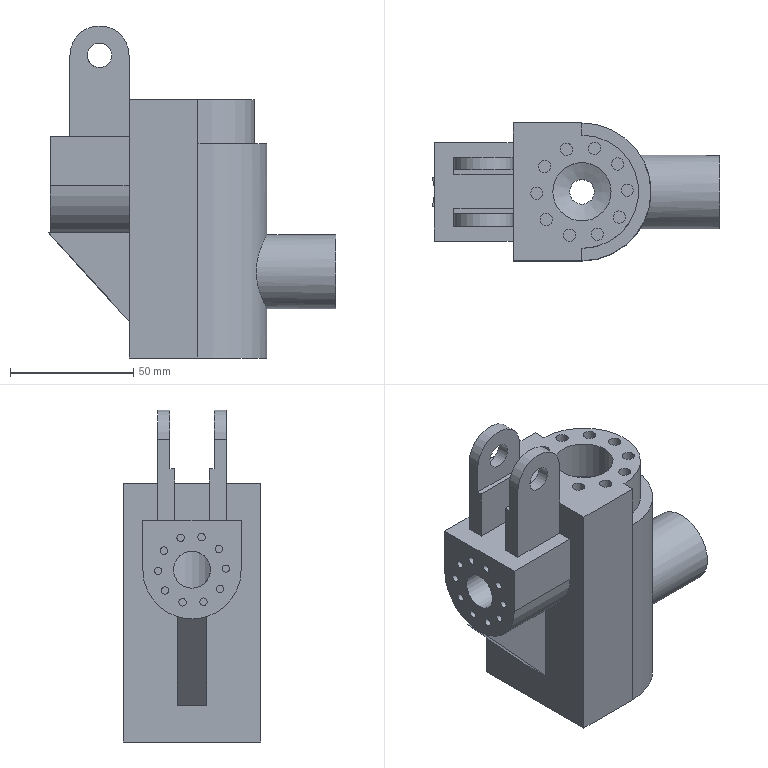Part | NX | features DATUM_CSYS 11, SKETCH 10, EXTRUDE 9, CYLINDER 8, BLEND 3, SYMBOLIC_THREAD 3, CHAMFER 2, CPROJ 2, UNITE 2, Container 1, EXTRACT_BODY 1, Geometry Instance 1, REPLACE_FACE 1 | 1 solid | 109 faces | box 116.842 x 56 x 135 mm | volume 278425 mm3 | plane 60 | cylinder 47 | cone 2 | commonest cylinder face diameters 3 x20 5 x10 40 x4 10 x3 15.016 x2 24 x2